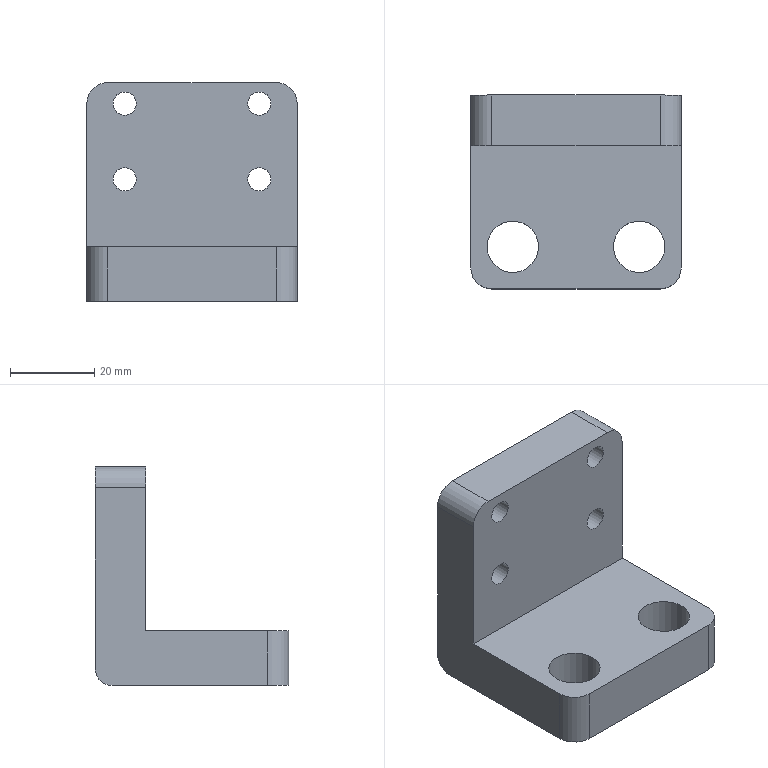Part | NX | features 切除-拉伸3 2 | 1 solid | 19 faces | box 50 x 46 x 52 mm | volume 48680 mm3 | cylinder 11 | plane 8 | commonest cylinder face diameters 5.5 x4 10 x4 12.2 x2 8 x1
STEP:
#1=CARTESIAN_POINT('',(-16.,123.3,71.75));
#2=VERTEX_POINT('',#1);
#3=CARTESIAN_POINT('',(-16.,123.3,74.5));
#4=DIRECTION('',(0.,-1.,0.));
#5=DIRECTION('',(0.,0.,-1.));
#6=AXIS2_PLACEMENT_3D('',#3,#4,#5);
#7=CIRCLE('',#6,2.75);
#8=EDGE_CURVE('',#2,#2,#7,.T.);
#9=ORIENTED_EDGE('',*,*,#8,.T.);
#10=EDGE_LOOP('',(#9));
#11=FACE_BOUND('',#10,.T.);
#12=CARTESIAN_POINT('',(-16.,135.3,71.75));
#13=VERTEX_POINT('',#12);
#14=CARTESIAN_POINT('',(-16.,135.3,74.5));
#15=DIRECTION('',(0.,-1.,0.));
#16=DIRECTION('',(0.,0.,-1.));
#17=AXIS2_PLACEMENT_3D('',#14,#15,#16);
#18=CIRCLE('',#17,2.75);
#19=EDGE_CURVE('',#13,#13,#18,.T.);
#20=ORIENTED_EDGE('',*,*,#19,.F.);
#21=EDGE_LOOP('',(#20));
#22=FACE_BOUND('',#21,.T.);
#23=CARTESIAN_POINT('',(-16.,135.3,74.5));
#24=DIRECTION('',(0.,-1.,0.));
#25=DIRECTION('',(-0.000000009,0.,-1.));
#26=AXIS2_PLACEMENT_3D('',#23,#24,#25);
#27=CYLINDRICAL_SURFACE('',#26,2.75);
#28=ADVANCED_FACE('',(#11,#22),#27,.F.);
#29=CARTESIAN_POINT('',(16.,123.3,71.75));
#30=VERTEX_POINT('',#29);
#31=CARTESIAN_POINT('',(16.,123.3,74.5));
#32=DIRECTION('',(0.,-1.,0.));
#33=DIRECTION('',(0.,0.,-1.));
#34=AXIS2_PLACEMENT_3D('',#31,#32,#33);
#35=CIRCLE('',#34,2.75);
#36=EDGE_CURVE('',#30,#30,#35,.T.);
#37=ORIENTED_EDGE('',*,*,#36,.T.);
#38=EDGE_LOOP('',(#37));
#39=FACE_BOUND('',#38,.T.);
#40=CARTESIAN_POINT('',(16.,135.3,71.75));
#41=VERTEX_POINT('',#40);
#42=CARTESIAN_POINT('',(16.,135.3,74.5));
#43=DIRECTION('',(0.,-1.,0.));
#44=DIRECTION('',(0.,0.,-1.));
#45=AXIS2_PLACEMENT_3D('',#42,#43,#44);
#46=CIRCLE('',#45,2.75);
#47=EDGE_CURVE('',#41,#41,#46,.T.);
#48=ORIENTED_EDGE('',*,*,#47,.F.);
#49=EDGE_LOOP('',(#48));
#50=FACE_BOUND('',#49,.T.);
#51=CARTESIAN_POINT('',(16.,135.3,74.5));
#52=DIRECTION('',(0.,-1.,0.));
#53=DIRECTION('',(-0.000000009,0.,-1.));
#54=AXIS2_PLACEMENT_3D('',#51,#52,#53);
#55=CYLINDRICAL_SURFACE('',#54,2.75);
#56=ADVANCED_FACE('',(#39,#50),#55,.F.);
#57=CARTESIAN_POINT('',(20.,89.3,45.5));
#58=VERTEX_POINT('',#57);
#59=CARTESIAN_POINT('',(-20.,89.3,45.5));
#60=VERTEX_POINT('',#59);
#61=CARTESIAN_POINT('',(-25.,89.3,45.5));
#62=DIRECTION('',(1.,0.,-0.000000009));
#63=VECTOR('',#62,1000.);
#64=LINE('',#61,#63);
#65=EDGE_CURVE('',#58,#60,#64,.F.);
#66=ORIENTED_EDGE('',*,*,#65,.F.);
#67=CARTESIAN_POINT('',(20.,89.3,58.5));
#68=VERTEX_POINT('',#67);
#69=CARTESIAN_POINT('',(20.,89.3,45.5));
#70=DIRECTION('',(-0.000000007,0.,-1.));
#71=VECTOR('',#70,1000.);
#72=LINE('',#69,#71);
#73=EDGE_CURVE('',#58,#68,#72,.F.);
#74=ORIENTED_EDGE('',*,*,#73,.T.);
#75=CARTESIAN_POINT('',(-20.,89.3,58.5));
#76=VERTEX_POINT('',#75);
#77=CARTESIAN_POINT('',(-25.,89.3,58.5));
#78=DIRECTION('',(-1.,0.,0.000000009));
#79=VECTOR('',#78,1000.);
#80=LINE('',#77,#79);
#81=EDGE_CURVE('',#68,#76,#80,.T.);
#82=ORIENTED_EDGE('',*,*,#81,.T.);
#83=CARTESIAN_POINT('',(-20.,89.3,45.5));
#84=DIRECTION('',(0.000000007,0.,1.));
#85=VECTOR('',#84,1000.);
#86=LINE('',#83,#85);
#87=EDGE_CURVE('',#76,#60,#86,.F.);
#88=ORIENTED_EDGE('',*,*,#87,.T.);
#89=EDGE_LOOP('',(#66,#74,#82,#88));
#90=FACE_BOUND('',#89,.T.);
#91=CARTESIAN_POINT('',(-25.,89.3,45.5));
#92=DIRECTION('',(0.,-1.,0.));
#93=DIRECTION('',(0.000000009,0.,1.));
#94=AXIS2_PLACEMENT_3D('',#91,#92,#93);
#95=PLANE('',#94);
#96=ADVANCED_FACE('',(#90),#95,.T.);
#97=CARTESIAN_POINT('',(-8.9,99.3,45.5));
#98=VERTEX_POINT('',#97);
#99=CARTESIAN_POINT('',(-15.,99.3,45.5));
#100=DIRECTION('',(0.000000009,0.,1.));
#101=DIRECTION('',(1.,0.,-0.000000009));
#102=AXIS2_PLACEMENT_3D('',#99,#100,#101);
#103=CIRCLE('',#102,6.1);
#104=EDGE_CURVE('',#98,#98,#103,.F.);
#105=ORIENTED_EDGE('',*,*,#104,.T.);
#106=EDGE_LOOP('',(#105));
#107=FACE_BOUND('',#106,.T.);
#108=CARTESIAN_POINT('',(-8.9,99.3,58.5));
#109=VERTEX_POINT('',#108);
#110=CARTESIAN_POINT('',(-15.,99.3,58.5));
#111=DIRECTION('',(0.000000009,0.,1.));
#112=DIRECTION('',(1.,0.,-0.000000009));
#113=AXIS2_PLACEMENT_3D('',#110,#111,#112);
#114=CIRCLE('',#113,6.1);
#115=EDGE_CURVE('',#109,#109,#114,.F.);
#116=ORIENTED_EDGE('',*,*,#115,.F.);
#117=EDGE_LOOP('',(#116));
#118=FACE_BOUND('',#117,.T.);
#119=CARTESIAN_POINT('',(-15.,99.3,-3.5));
#120=DIRECTION('',(-0.000000009,0.,-1.));
#121=DIRECTION('',(0.,1.,0.));
#122=AXIS2_PLACEMENT_3D('',#119,#120,#121);
#123=CYLINDRICAL_SURFACE('',#122,6.1);
#124=ADVANCED_FACE('',(#107,#118),#123,.F.);
#125=CARTESIAN_POINT('',(21.1,99.3,45.5));
#126=VERTEX_POINT('',#125);
#127=CARTESIAN_POINT('',(15.,99.3,45.5));
#128=DIRECTION('',(0.000000009,0.,1.));
#129=DIRECTION('',(1.,0.,-0.000000009));
#130=AXIS2_PLACEMENT_3D('',#127,#128,#129);
#131=CIRCLE('',#130,6.1);
#132=EDGE_CURVE('',#126,#126,#131,.F.);
#133=ORIENTED_EDGE('',*,*,#132,.T.);
#134=EDGE_LOOP('',(#133));
#135=FACE_BOUND('',#134,.T.);
#136=CARTESIAN_POINT('',(21.1,99.3,58.5));
#137=VERTEX_POINT('',#136);
#138=CARTESIAN_POINT('',(15.,99.3,58.5));
#139=DIRECTION('',(0.000000009,0.,1.));
#140=DIRECTION('',(1.,0.,-0.000000009));
#141=AXIS2_PLACEMENT_3D('',#138,#139,#140);
#142=CIRCLE('',#141,6.1);
#143=EDGE_CURVE('',#137,#137,#142,.F.);
#144=ORIENTED_EDGE('',*,*,#143,.F.);
#145=EDGE_LOOP('',(#144));
#146=FACE_BOUND('',#145,.T.);
#147=CARTESIAN_POINT('',(15.,99.3,-3.5));
#148=DIRECTION('',(-0.000000009,0.,-1.));
#149=DIRECTION('',(0.,1.,0.));
#150=AXIS2_PLACEMENT_3D('',#147,#148,#149);
#151=CYLINDRICAL_SURFACE('',#150,6.1);
#152=ADVANCED_FACE('',(#135,#146),#151,.F.);
#153=CARTESIAN_POINT('',(25.,94.3,45.5));
#154=VERTEX_POINT('',#153);
#155=CARTESIAN_POINT('',(20.,94.3,45.5));
#156=DIRECTION('',(0.000000007,0.,1.));
#157=DIRECTION('',(0.,-1.,0.));
#158=AXIS2_PLACEMENT_3D('',#155,#156,#157);
#159=CIRCLE('',#158,5.);
#160=EDGE_CURVE('',#154,#58,#159,.F.);
#161=ORIENTED_EDGE('',*,*,#160,.F.);
#162=CARTESIAN_POINT('',(25.,94.3,58.5));
#163=VERTEX_POINT('',#162);
#164=CARTESIAN_POINT('',(25.,94.3,47.5));
#165=DIRECTION('',(0.000000007,0.,1.));
#166=VECTOR('',#165,1000.);
#167=LINE('',#164,#166);
#168=EDGE_CURVE('',#163,#154,#167,.F.);
#169=ORIENTED_EDGE('',*,*,#168,.F.);
#170=CARTESIAN_POINT('',(20.,94.3,58.5));
#171=DIRECTION('',(0.000000009,0.,1.));
#172=DIRECTION('',(1.,0.,-0.000000009));
#173=AXIS2_PLACEMENT_3D('',#170,#171,#172);
#174=CIRCLE('',#173,5.);
#175=EDGE_CURVE('',#68,#163,#174,.T.);
#176=ORIENTED_EDGE('',*,*,#175,.F.);
#177=ORIENTED_EDGE('',*,*,#73,.F.);
#178=EDGE_LOOP('',(#161,#169,#176,#177));
#179=FACE_BOUND('',#178,.T.);
#180=CARTESIAN_POINT('',(20.,94.3,49.5));
#181=DIRECTION('',(-0.000000007,0.,-1.));
#182=DIRECTION('',(1.,0.,-0.000000007));
#183=AXIS2_PLACEMENT_3D('',#180,#181,#182);
#184=CYLINDRICAL_SURFACE('',#183,5.);
#185=ADVANCED_FACE('',(#179),#184,.T.);
#186=CARTESIAN_POINT('',(-25.,94.3,45.5));
#187=VERTEX_POINT('',#186);
#188=CARTESIAN_POINT('',(-20.,94.3,45.5));
#189=DIRECTION('',(0.000000007,0.,1.));
#190=DIRECTION('',(0.,-1.,0.));
#191=AXIS2_PLACEMENT_3D('',#188,#189,#190);
#192=CIRCLE('',#191,5.);
#193=EDGE_CURVE('',#60,#187,#192,.F.);
#194=ORIENTED_EDGE('',*,*,#193,.F.);
#195=ORIENTED_EDGE('',*,*,#87,.F.);
#196=CARTESIAN_POINT('',(-25.,94.3,58.5));
#197=VERTEX_POINT('',#196);
#198=CARTESIAN_POINT('',(-20.,94.3,58.5));
#199=DIRECTION('',(0.000000009,0.,1.));
#200=DIRECTION('',(1.,0.,-0.000000009));
#201=AXIS2_PLACEMENT_3D('',#198,#199,#200);
#202=CIRCLE('',#201,5.);
#203=EDGE_CURVE('',#197,#76,#202,.T.);
#204=ORIENTED_EDGE('',*,*,#203,.F.);
#205=CARTESIAN_POINT('',(-25.,94.3,49.5));
#206=DIRECTION('',(-0.000000007,0.,-1.));
#207=VECTOR('',#206,1000.);
#208=LINE('',#205,#207);
#209=EDGE_CURVE('',#187,#197,#208,.F.);
#210=ORIENTED_EDGE('',*,*,#209,.F.);
#211=EDGE_LOOP('',(#194,#195,#204,#210));
#212=FACE_BOUND('',#211,.T.);
#213=CARTESIAN_POINT('',(-20.,94.3,45.5));
#214=DIRECTION('',(0.000000007,0.,1.));
#215=DIRECTION('',(-1.,0.,0.000000007));
#216=AXIS2_PLACEMENT_3D('',#213,#214,#215);
#217=CYLINDRICAL_SURFACE('',#216,5.);
#218=ADVANCED_FACE('',(#212),#217,.T.);
#219=ORIENTED_EDGE('',*,*,#132,.F.);
#220=EDGE_LOOP('',(#219));
#221=FACE_BOUND('',#220,.T.);
#222=ORIENTED_EDGE('',*,*,#104,.F.);
#223=EDGE_LOOP('',(#222));
#224=FACE_BOUND('',#223,.T.);
#225=CARTESIAN_POINT('',(-25.,131.3,45.5));
#226=VERTEX_POINT('',#225);
#227=CARTESIAN_POINT('',(-25.,89.3,45.5));
#228=DIRECTION('',(0.,1.,0.));
#229=VECTOR('',#228,1000.);
#230=LINE('',#227,#229);
#231=EDGE_CURVE('',#226,#187,#230,.F.);
#232=ORIENTED_EDGE('',*,*,#231,.F.);
#233=CARTESIAN_POINT('',(25.,131.3,45.5));
#234=VERTEX_POINT('',#233);
#235=CARTESIAN_POINT('',(-25.,131.3,45.5));
#236=DIRECTION('',(1.,0.,-0.000000009));
#237=VECTOR('',#236,1000.);
#238=LINE('',#235,#237);
#239=EDGE_CURVE('',#234,#226,#238,.F.);
#240=ORIENTED_EDGE('',*,*,#239,.F.);
#241=CARTESIAN_POINT('',(25.,89.3,45.5));
#242=DIRECTION('',(0.,1.,0.));
#243=VECTOR('',#242,1000.);
#244=LINE('',#241,#243);
#245=EDGE_CURVE('',#234,#154,#244,.F.);
#246=ORIENTED_EDGE('',*,*,#245,.T.);
#247=ORIENTED_EDGE('',*,*,#160,.T.);
#248=ORIENTED_EDGE('',*,*,#65,.T.);
#249=ORIENTED_EDGE('',*,*,#193,.T.);
#250=EDGE_LOOP('',(#232,#240,#246,#247,#248,#249));
#251=FACE_BOUND('',#250,.T.);
#252=CARTESIAN_POINT('',(-25.,89.3,45.5));
#253=DIRECTION('',(0.000000009,0.,1.));
#254=DIRECTION('',(0.,1.,0.));
#255=AXIS2_PLACEMENT_3D('',#252,#253,#254);
#256=PLANE('',#255);
#257=ADVANCED_FACE('',(#221,#224,#251),#256,.F.);
#258=CARTESIAN_POINT('',(-16.,123.3,89.75));
#259=VERTEX_POINT('',#258);
#260=CARTESIAN_POINT('',(-16.,123.3,92.5));
#261=DIRECTION('',(0.,-1.,0.));
#262=DIRECTION('',(0.,0.,-1.));
#263=AXIS2_PLACEMENT_3D('',#260,#261,#262);
#264=CIRCLE('',#263,2.75);
#265=EDGE_CURVE('',#259,#259,#264,.T.);
#266=ORIENTED_EDGE('',*,*,#265,.T.);
#267=EDGE_LOOP('',(#266));
#268=FACE_BOUND('',#267,.T.);
#269=CARTESIAN_POINT('',(-16.,135.3,89.75));
#270=VERTEX_POINT('',#269);
#271=CARTESIAN_POINT('',(-16.,135.3,92.5));
#272=DIRECTION('',(0.,1.,0.));
#273=DIRECTION('',(-0.000000009,0.,-1.));
#274=AXIS2_PLACEMENT_3D('',#271,#272,#273);
#275=CIRCLE('',#274,2.75);
#276=EDGE_CURVE('',#270,#270,#275,.F.);
#277=ORIENTED_EDGE('',*,*,#276,.F.);
#278=EDGE_LOOP('',(#277));
#279=FACE_BOUND('',#278,.T.);
#280=CARTESIAN_POINT('',(-16.,135.3,92.5));
#281=DIRECTION('',(0.,-1.,0.));
#282=DIRECTION('',(0.000000009,0.,1.));
#283=AXIS2_PLACEMENT_3D('',#280,#281,#282);
#284=CYLINDRICAL_SURFACE('',#283,2.75);
#285=ADVANCED_FACE('',(#268,#279),#284,.F.);
#286=CARTESIAN_POINT('',(16.,123.3,89.75));
#287=VERTEX_POINT('',#286);
#288=CARTESIAN_POINT('',(16.,123.3,92.5));
#289=DIRECTION('',(0.,-1.,0.));
#290=DIRECTION('',(0.,0.,-1.));
#291=AXIS2_PLACEMENT_3D('',#288,#289,#290);
#292=CIRCLE('',#291,2.75);
#293=EDGE_CURVE('',#287,#287,#292,.T.);
#294=ORIENTED_EDGE('',*,*,#293,.T.);
#295=EDGE_LOOP('',(#294));
#296=FACE_BOUND('',#295,.T.);
#297=CARTESIAN_POINT('',(16.,135.3,89.75));
#298=VERTEX_POINT('',#297);
#299=CARTESIAN_POINT('',(16.,135.3,92.5));
#300=DIRECTION('',(0.,1.,0.));
#301=DIRECTION('',(-0.000000009,0.,-1.));
#302=AXIS2_PLACEMENT_3D('',#299,#300,#301);
#303=CIRCLE('',#302,2.75);
#304=EDGE_CURVE('',#298,#298,#303,.F.);
#305=ORIENTED_EDGE('',*,*,#304,.F.);
#306=EDGE_LOOP('',(#305));
#307=FACE_BOUND('',#306,.T.);
#308=CARTESIAN_POINT('',(16.,135.3,92.5));
#309=DIRECTION('',(0.,-1.,0.));
#310=DIRECTION('',(0.000000009,0.,1.));
#311=AXIS2_PLACEMENT_3D('',#308,#309,#310);
#312=CYLINDRICAL_SURFACE('',#311,2.75);
#313=ADVANCED_FACE('',(#296,#307),#312,.F.);
#314=CARTESIAN_POINT('',(25.,123.3,92.5));
#315=VERTEX_POINT('',#314);
#316=CARTESIAN_POINT('',(25.,123.3,58.5));
#317=VERTEX_POINT('',#316);
#318=CARTESIAN_POINT('',(25.,123.3,49.5));
#319=DIRECTION('',(-0.000000007,0.,-1.));
#320=VECTOR('',#319,1000.);
#321=LINE('',#318,#320);
#322=EDGE_CURVE('',#315,#317,#321,.T.);
#323=ORIENTED_EDGE('',*,*,#322,.T.);
#324=CARTESIAN_POINT('',(25.,135.3,58.5));
#325=DIRECTION('',(0.,-1.,0.));
#326=VECTOR('',#325,1000.);
#327=LINE('',#324,#326);
#328=EDGE_CURVE('',#317,#163,#327,.T.);
#329=ORIENTED_EDGE('',*,*,#328,.T.);
#330=ORIENTED_EDGE('',*,*,#168,.T.);
#331=ORIENTED_EDGE('',*,*,#245,.F.);
#332=CARTESIAN_POINT('',(25.,135.3,49.5));
#333=VERTEX_POINT('',#332);
#334=CARTESIAN_POINT('',(25.,131.3,49.5));
#335=DIRECTION('',(1.,0.,-0.000000007));
#336=DIRECTION('',(-0.000000007,0.,-1.));
#337=AXIS2_PLACEMENT_3D('',#334,#335,#336);
#338=CIRCLE('',#337,4.);
#339=EDGE_CURVE('',#333,#234,#338,.F.);
#340=ORIENTED_EDGE('',*,*,#339,.F.);
#341=CARTESIAN_POINT('',(25.,135.3,92.5));
#342=VERTEX_POINT('',#341);
#343=CARTESIAN_POINT('',(25.,135.3,45.5));
#344=DIRECTION('',(0.000000007,0.,1.));
#345=VECTOR('',#344,1000.);
#346=LINE('',#343,#345);
#347=EDGE_CURVE('',#342,#333,#346,.F.);
#348=ORIENTED_EDGE('',*,*,#347,.F.);
#349=CARTESIAN_POINT('',(25.,135.3,92.5));
#350=DIRECTION('',(0.,-1.,0.));
#351=VECTOR('',#350,1000.);
#352=LINE('',#349,#351);
#353=EDGE_CURVE('',#342,#315,#352,.T.);
#354=ORIENTED_EDGE('',*,*,#353,.T.);
#355=EDGE_LOOP('',(#323,#329,#330,#331,#340,#348,#354));
#356=FACE_BOUND('',#355,.T.);
#357=CARTESIAN_POINT('',(25.,135.3,49.5));
#358=DIRECTION('',(1.,0.,-0.000000007));
#359=DIRECTION('',(0.000000007,0.,1.));
#360=AXIS2_PLACEMENT_3D('',#357,#358,#359);
#361=PLANE('',#360);
#362=ADVANCED_FACE('',(#356),#361,.T.);
#363=CARTESIAN_POINT('',(20.,123.3,97.5));
#364=VERTEX_POINT('',#363);
#365=CARTESIAN_POINT('',(20.,123.3,92.5));
#366=DIRECTION('',(0.,-1.,0.));
#367=DIRECTION('',(0.,0.,-1.));
#368=AXIS2_PLACEMENT_3D('',#365,#366,#367);
#369=CIRCLE('',#368,5.);
#370=EDGE_CURVE('',#315,#364,#369,.T.);
#371=ORIENTED_EDGE('',*,*,#370,.F.);
#372=ORIENTED_EDGE('',*,*,#353,.F.);
#373=CARTESIAN_POINT('',(20.,135.3,97.5));
#374=VERTEX_POINT('',#373);
#375=CARTESIAN_POINT('',(20.,135.3,92.5));
#376=DIRECTION('',(0.,-1.,0.));
#377=DIRECTION('',(0.,0.,-1.));
#378=AXIS2_PLACEMENT_3D('',#375,#376,#377);
#379=CIRCLE('',#378,5.);
#380=EDGE_CURVE('',#374,#342,#379,.F.);
#381=ORIENTED_EDGE('',*,*,#380,.F.);
#382=CARTESIAN_POINT('',(20.,133.3,97.5));
#383=DIRECTION('',(0.,-1.,0.));
#384=VECTOR('',#383,1000.);
#385=LINE('',#382,#384);
#386=EDGE_CURVE('',#364,#374,#385,.F.);
#387=ORIENTED_EDGE('',*,*,#386,.F.);
#388=EDGE_LOOP('',(#371,#372,#381,#387));
#389=FACE_BOUND('',#388,.T.);
#390=CARTESIAN_POINT('',(20.,135.3,92.5));
#391=DIRECTION('',(0.,-1.,0.));
#392=DIRECTION('',(0.,0.,-1.));
#393=AXIS2_PLACEMENT_3D('',#390,#391,#392);
#394=CYLINDRICAL_SURFACE('',#393,5.);
#395=ADVANCED_FACE('',(#389),#394,.T.);
#396=CARTESIAN_POINT('',(-20.,123.3,97.5));
#397=VERTEX_POINT('',#396);
#398=CARTESIAN_POINT('',(-25.,123.3,97.5));
#399=DIRECTION('',(-1.,0.,0.000000009));
#400=VECTOR('',#399,1000.);
#401=LINE('',#398,#400);
#402=EDGE_CURVE('',#364,#397,#401,.T.);
#403=ORIENTED_EDGE('',*,*,#402,.F.);
#404=ORIENTED_EDGE('',*,*,#386,.T.);
#405=CARTESIAN_POINT('',(-20.,135.3,97.5));
#406=VERTEX_POINT('',#405);
#407=CARTESIAN_POINT('',(-25.,135.3,97.5));
#408=DIRECTION('',(1.,0.,-0.000000009));
#409=VECTOR('',#408,1000.);
#410=LINE('',#407,#409);
#411=EDGE_CURVE('',#374,#406,#410,.F.);
#412=ORIENTED_EDGE('',*,*,#411,.T.);
#413=CARTESIAN_POINT('',(-20.,133.3,97.5));
#414=DIRECTION('',(0.,-1.,0.));
#415=VECTOR('',#414,1000.);
#416=LINE('',#413,#415);
#417=EDGE_CURVE('',#406,#397,#416,.T.);
#418=ORIENTED_EDGE('',*,*,#417,.T.);
#419=EDGE_LOOP('',(#403,#404,#412,#418));
#420=FACE_BOUND('',#419,.T.);
#421=CARTESIAN_POINT('',(-25.,133.3,97.5));
#422=DIRECTION('',(0.000000009,0.,1.));
#423=DIRECTION('',(-1.,0.,0.000000009));
#424=AXIS2_PLACEMENT_3D('',#421,#422,#423);
#425=PLANE('',#424);
#426=ADVANCED_FACE('',(#420),#425,.T.);
#427=CARTESIAN_POINT('',(-25.,123.3,92.5));
#428=VERTEX_POINT('',#427);
#429=CARTESIAN_POINT('',(-20.,123.3,92.5));
#430=DIRECTION('',(0.,-1.,0.));
#431=DIRECTION('',(0.,0.,-1.));
#432=AXIS2_PLACEMENT_3D('',#429,#430,#431);
#433=CIRCLE('',#432,5.);
#434=EDGE_CURVE('',#397,#428,#433,.T.);
#435=ORIENTED_EDGE('',*,*,#434,.F.);
#436=ORIENTED_EDGE('',*,*,#417,.F.);
#437=CARTESIAN_POINT('',(-25.,135.3,92.5));
#438=VERTEX_POINT('',#437);
#439=CARTESIAN_POINT('',(-20.,135.3,92.5));
#440=DIRECTION('',(0.,-1.,0.));
#441=DIRECTION('',(0.,0.,-1.));
#442=AXIS2_PLACEMENT_3D('',#439,#440,#441);
#443=CIRCLE('',#442,5.);
#444=EDGE_CURVE('',#438,#406,#443,.F.);
#445=ORIENTED_EDGE('',*,*,#444,.F.);
#446=CARTESIAN_POINT('',(-25.,131.3,92.5));
#447=DIRECTION('',(0.,-1.,0.));
#448=VECTOR('',#447,1000.);
#449=LINE('',#446,#448);
#450=EDGE_CURVE('',#428,#438,#449,.F.);
#451=ORIENTED_EDGE('',*,*,#450,.F.);
#452=EDGE_LOOP('',(#435,#436,#445,#451));
#453=FACE_BOUND('',#452,.T.);
#454=CARTESIAN_POINT('',(-20.,133.3,92.5));
#455=DIRECTION('',(0.,-1.,0.));
#456=DIRECTION('',(0.,0.,-1.));
#457=AXIS2_PLACEMENT_3D('',#454,#455,#456);
#458=CYLINDRICAL_SURFACE('',#457,5.);
#459=ADVANCED_FACE('',(#453),#458,.T.);
#460=CARTESIAN_POINT('',(-25.,135.3,49.5));
#461=VERTEX_POINT('',#460);
#462=CARTESIAN_POINT('',(-25.,135.3,45.5));
#463=DIRECTION('',(0.000000007,0.,1.));
#464=VECTOR('',#463,1000.);
#465=LINE('',#462,#464);
#466=EDGE_CURVE('',#438,#461,#465,.F.);
#467=ORIENTED_EDGE('',*,*,#466,.T.);
#468=CARTESIAN_POINT('',(-25.,131.3,49.5));
#469=DIRECTION('',(1.,0.,-0.000000007));
#470=DIRECTION('',(-0.000000007,0.,-1.));
#471=AXIS2_PLACEMENT_3D('',#468,#469,#470);
#472=CIRCLE('',#471,4.);
#473=EDGE_CURVE('',#461,#226,#472,.F.);
#474=ORIENTED_EDGE('',*,*,#473,.T.);
#475=ORIENTED_EDGE('',*,*,#231,.T.);
#476=ORIENTED_EDGE('',*,*,#209,.T.);
#477=CARTESIAN_POINT('',(-25.,123.3,58.5));
#478=VERTEX_POINT('',#477);
#479=CARTESIAN_POINT('',(-25.,89.3,58.5));
#480=DIRECTION('',(0.,-1.,0.));
#481=VECTOR('',#480,1000.);
#482=LINE('',#479,#481);
#483=EDGE_CURVE('',#478,#197,#482,.T.);
#484=ORIENTED_EDGE('',*,*,#483,.F.);
#485=CARTESIAN_POINT('',(-25.,123.3,45.5));
#486=DIRECTION('',(-0.000000007,0.,-1.));
#487=VECTOR('',#486,1000.);
#488=LINE('',#485,#487);
#489=EDGE_CURVE('',#428,#478,#488,.T.);
#490=ORIENTED_EDGE('',*,*,#489,.F.);
#491=ORIENTED_EDGE('',*,*,#450,.T.);
#492=EDGE_LOOP('',(#467,#474,#475,#476,#484,#490,#491));
#493=FACE_BOUND('',#492,.T.);
#494=CARTESIAN_POINT('',(-25.,131.3,45.5));
#495=DIRECTION('',(-1.,0.,0.000000007));
#496=DIRECTION('',(-0.000000007,0.,-1.));
#497=AXIS2_PLACEMENT_3D('',#494,#495,#496);
#498=PLANE('',#497);
#499=ADVANCED_FACE('',(#493),#498,.T.);
#500=ORIENTED_EDGE('',*,*,#339,.T.);
#501=ORIENTED_EDGE('',*,*,#239,.T.);
#502=ORIENTED_EDGE('',*,*,#473,.F.);
#503=CARTESIAN_POINT('',(-25.,135.3,49.5));
#504=DIRECTION('',(1.,0.,-0.000000009));
#505=VECTOR('',#504,1000.);
#506=LINE('',#503,#505);
#507=EDGE_CURVE('',#333,#461,#506,.F.);
#508=ORIENTED_EDGE('',*,*,#507,.F.);
#509=EDGE_LOOP('',(#500,#501,#502,#508));
#510=FACE_BOUND('',#509,.T.);
#511=CARTESIAN_POINT('',(-25.,131.3,49.5));
#512=DIRECTION('',(1.,0.,-0.000000009));
#513=DIRECTION('',(0.000000009,0.,1.));
#514=AXIS2_PLACEMENT_3D('',#511,#512,#513);
#515=CYLINDRICAL_SURFACE('',#514,4.);
#516=ADVANCED_FACE('',(#510),#515,.T.);
#517=ORIENTED_EDGE('',*,*,#19,.T.);
#518=EDGE_LOOP('',(#517));
#519=FACE_BOUND('',#518,.T.);
#520=ORIENTED_EDGE('',*,*,#47,.T.);
#521=EDGE_LOOP('',(#520));
#522=FACE_BOUND('',#521,.T.);
#523=ORIENTED_EDGE('',*,*,#507,.T.);
#524=ORIENTED_EDGE('',*,*,#466,.F.);
#525=ORIENTED_EDGE('',*,*,#444,.T.);
#526=ORIENTED_EDGE('',*,*,#411,.F.);
#527=ORIENTED_EDGE('',*,*,#380,.T.);
#528=ORIENTED_EDGE('',*,*,#347,.T.);
#529=EDGE_LOOP('',(#523,#524,#525,#526,#527,#528));
#530=FACE_BOUND('',#529,.T.);
#531=ORIENTED_EDGE('',*,*,#304,.T.);
#532=EDGE_LOOP('',(#531));
#533=FACE_BOUND('',#532,.T.);
#534=ORIENTED_EDGE('',*,*,#276,.T.);
#535=EDGE_LOOP('',(#534));
#536=FACE_BOUND('',#535,.T.);
#537=CARTESIAN_POINT('',(-25.,135.3,45.5));
#538=DIRECTION('',(0.,-1.,0.));
#539=DIRECTION('',(0.000000009,0.,1.));
#540=AXIS2_PLACEMENT_3D('',#537,#538,#539);
#541=PLANE('',#540);
#542=ADVANCED_FACE('',(#519,#522,#530,#533,#536),#541,.F.);
#543=ORIENTED_EDGE('',*,*,#143,.T.);
#544=EDGE_LOOP('',(#543));
#545=FACE_BOUND('',#544,.T.);
#546=ORIENTED_EDGE('',*,*,#115,.T.);
#547=EDGE_LOOP('',(#546));
#548=FACE_BOUND('',#547,.T.);
#549=ORIENTED_EDGE('',*,*,#328,.F.);
#550=CARTESIAN_POINT('',(-25.,123.3,58.5));
#551=DIRECTION('',(-1.,0.,0.000000009));
#552=VECTOR('',#551,1000.);
#553=LINE('',#550,#552);
#554=EDGE_CURVE('',#317,#478,#553,.T.);
#555=ORIENTED_EDGE('',*,*,#554,.T.);
#556=ORIENTED_EDGE('',*,*,#483,.T.);
#557=ORIENTED_EDGE('',*,*,#203,.T.);
#558=ORIENTED_EDGE('',*,*,#81,.F.);
#559=ORIENTED_EDGE('',*,*,#175,.T.);
#560=EDGE_LOOP('',(#549,#555,#556,#557,#558,#559));
#561=FACE_BOUND('',#560,.T.);
#562=CARTESIAN_POINT('',(-25.,89.3,58.5));
#563=DIRECTION('',(0.000000009,0.,1.));
#564=DIRECTION('',(0.,1.,0.));
#565=AXIS2_PLACEMENT_3D('',#562,#563,#564);
#566=PLANE('',#565);
#567=ADVANCED_FACE('',(#545,#548,#561),#566,.T.);
#568=ORIENTED_EDGE('',*,*,#8,.F.);
#569=EDGE_LOOP('',(#568));
#570=FACE_BOUND('',#569,.T.);
#571=ORIENTED_EDGE('',*,*,#36,.F.);
#572=EDGE_LOOP('',(#571));
#573=FACE_BOUND('',#572,.T.);
#574=ORIENTED_EDGE('',*,*,#554,.F.);
#575=ORIENTED_EDGE('',*,*,#322,.F.);
#576=ORIENTED_EDGE('',*,*,#370,.T.);
#577=ORIENTED_EDGE('',*,*,#402,.T.);
#578=ORIENTED_EDGE('',*,*,#434,.T.);
#579=ORIENTED_EDGE('',*,*,#489,.T.);
#580=EDGE_LOOP('',(#574,#575,#576,#577,#578,#579));
#581=FACE_BOUND('',#580,.T.);
#582=ORIENTED_EDGE('',*,*,#293,.F.);
#583=EDGE_LOOP('',(#582));
#584=FACE_BOUND('',#583,.T.);
#585=ORIENTED_EDGE('',*,*,#265,.F.);
#586=EDGE_LOOP('',(#585));
#587=FACE_BOUND('',#586,.T.);
#588=CARTESIAN_POINT('',(-25.,123.3,45.5));
#589=DIRECTION('',(0.,-1.,0.));
#590=DIRECTION('',(0.000000009,0.,1.));
#591=AXIS2_PLACEMENT_3D('',#588,#589,#590);
#592=PLANE('',#591);
#593=ADVANCED_FACE('',(#570,#573,#581,#584,#587),#592,.T.);
#594=CLOSED_SHELL('',(#28,#56,#96,#124,#152,#185,#218,#257,#285,#313,#362,#395,#426,#459,#499,#516,#542,#567,#593));
#595=MANIFOLD_SOLID_BREP('',#594);
#596=(LENGTH_UNIT()NAMED_UNIT(*)SI_UNIT(.MILLI.,.METRE.));
#597=UNCERTAINTY_MEASURE_WITH_UNIT(LENGTH_MEASURE(0.00001),#596,'','');
#598=(NAMED_UNIT(*)PLANE_ANGLE_UNIT()SI_UNIT($,.RADIAN.));
#599=(NAMED_UNIT(*)SI_UNIT($,.STERADIAN.)SOLID_ANGLE_UNIT());
#600=(GEOMETRIC_REPRESENTATION_CONTEXT(3)GLOBAL_UNCERTAINTY_ASSIGNED_CONTEXT((#597))GLOBAL_UNIT_ASSIGNED_CONTEXT((#596,#598,#599))REPRESENTATION_CONTEXT('',''));
#601=ADVANCED_BREP_SHAPE_REPRESENTATION('',(#595),#600);